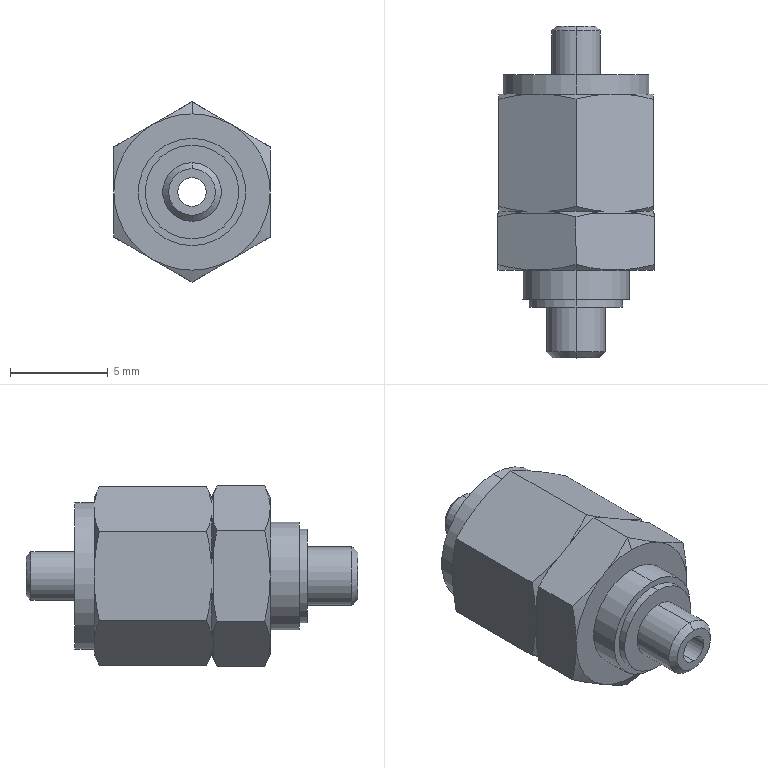Part | STEP file | BKC0425-M3 | 1 solid | 79 faces | box 8 x 17 x 9.238 mm | volume 562.812 mm3 | cone 33 | plane 28 | cylinder 18 | commonest cylinder face diameters 3 x4 1.463 x2 1.5 x2 2.5 x2 4 x2 4.8 x2